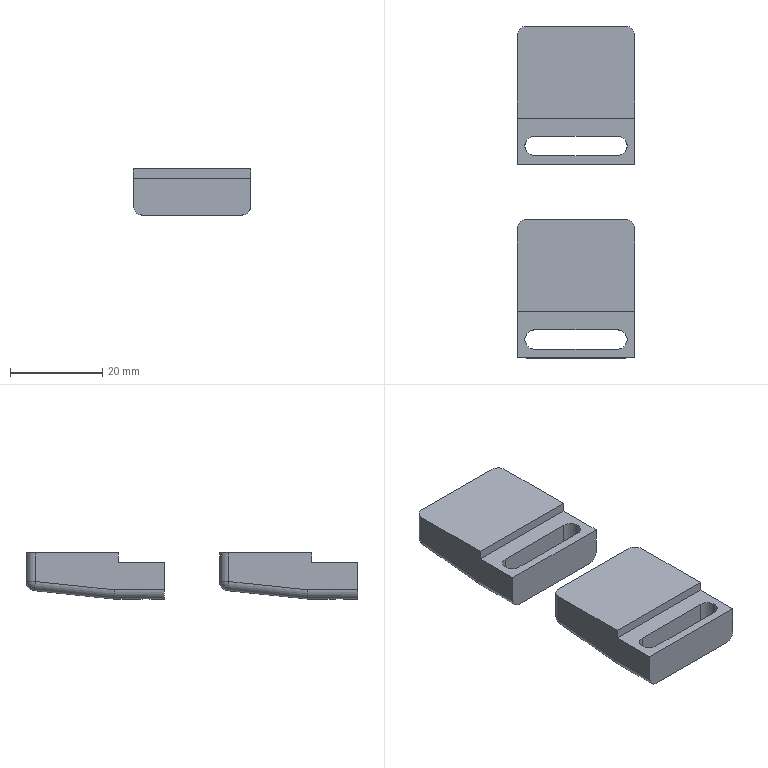Part | 2 solids | 54 faces | box 25.5 x 72 x 10 mm | volume 10910 mm3 | plane 28 | cylinder 22 | sphere 4 | commonest cylinder face diameters 4 x16 4.2 x4 10 x2